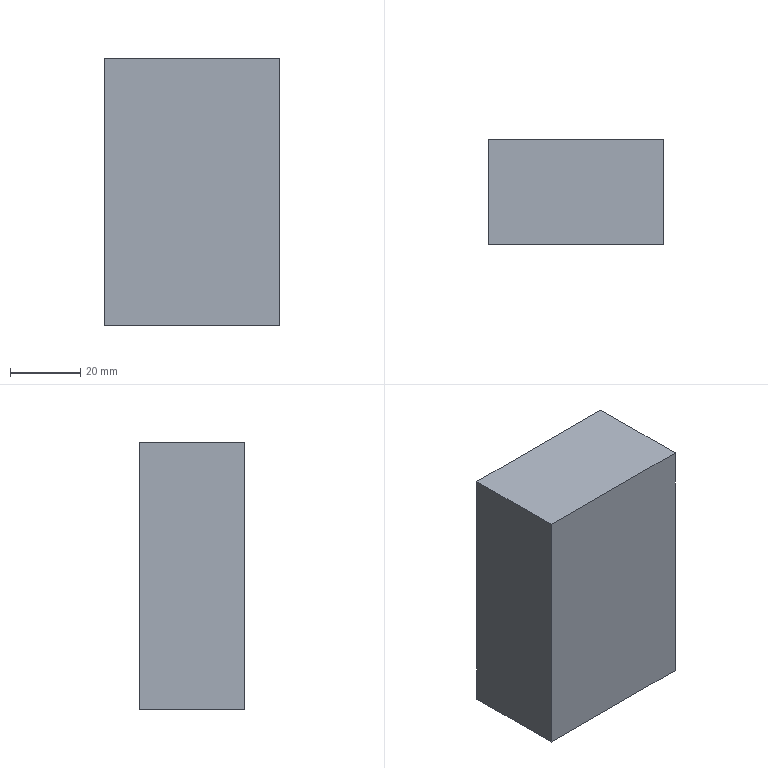Part | SolidWorks | features Extrusion 1 | 1 solid | 6 faces | box 50 x 30 x 76 mm | volume 114000 mm3 | plane 6
STEP:
#1=CARTESIAN_POINT('',(-25.,15.,0.));
#2=VERTEX_POINT('',#1);
#3=CARTESIAN_POINT('',(-25.,-15.,0.));
#4=VERTEX_POINT('',#3);
#5=CARTESIAN_POINT('',(-25.,-15.,0.));
#6=DIRECTION('',(0.,-1.,0.));
#7=VECTOR('',#6,1000.);
#8=LINE('',#5,#7);
#9=EDGE_CURVE('',#2,#4,#8,.T.);
#10=ORIENTED_EDGE('',*,*,#9,.T.);
#11=CARTESIAN_POINT('',(-25.,-15.,76.));
#12=VERTEX_POINT('',#11);
#13=CARTESIAN_POINT('',(-25.,-15.,76.));
#14=DIRECTION('',(0.,0.,-1.));
#15=VECTOR('',#14,1000.);
#16=LINE('',#13,#15);
#17=EDGE_CURVE('',#12,#4,#16,.T.);
#18=ORIENTED_EDGE('',*,*,#17,.F.);
#19=CARTESIAN_POINT('',(-25.,15.,76.));
#20=VERTEX_POINT('',#19);
#21=CARTESIAN_POINT('',(-25.,-15.,76.));
#22=DIRECTION('',(0.,-1.,0.));
#23=VECTOR('',#22,1000.);
#24=LINE('',#21,#23);
#25=EDGE_CURVE('',#20,#12,#24,.T.);
#26=ORIENTED_EDGE('',*,*,#25,.F.);
#27=CARTESIAN_POINT('',(-25.,15.,76.));
#28=DIRECTION('',(0.,0.,-1.));
#29=VECTOR('',#28,1000.);
#30=LINE('',#27,#29);
#31=EDGE_CURVE('',#20,#2,#30,.T.);
#32=ORIENTED_EDGE('',*,*,#31,.T.);
#33=EDGE_LOOP('',(#10,#18,#26,#32));
#34=FACE_OUTER_BOUND('',#33,.T.);
#35=CARTESIAN_POINT('',(-25.,-15.,76.));
#36=DIRECTION('',(1.,0.,0.));
#37=DIRECTION('',(0.,0.,-1.));
#38=AXIS2_PLACEMENT_3D('',#35,#36,#37);
#39=PLANE('',#38);
#40=ADVANCED_FACE('',(#34),#39,.F.);
#41=CARTESIAN_POINT('',(25.,-15.,0.));
#42=VERTEX_POINT('',#41);
#43=CARTESIAN_POINT('',(25.,-15.,0.));
#44=DIRECTION('',(1.,0.,0.));
#45=VECTOR('',#44,1000.);
#46=LINE('',#43,#45);
#47=EDGE_CURVE('',#4,#42,#46,.T.);
#48=ORIENTED_EDGE('',*,*,#47,.T.);
#49=CARTESIAN_POINT('',(25.,-15.,76.));
#50=VERTEX_POINT('',#49);
#51=CARTESIAN_POINT('',(25.,-15.,76.));
#52=DIRECTION('',(0.,0.,-1.));
#53=VECTOR('',#52,1000.);
#54=LINE('',#51,#53);
#55=EDGE_CURVE('',#50,#42,#54,.T.);
#56=ORIENTED_EDGE('',*,*,#55,.F.);
#57=CARTESIAN_POINT('',(25.,-15.,76.));
#58=DIRECTION('',(1.,0.,0.));
#59=VECTOR('',#58,1000.);
#60=LINE('',#57,#59);
#61=EDGE_CURVE('',#12,#50,#60,.T.);
#62=ORIENTED_EDGE('',*,*,#61,.F.);
#63=ORIENTED_EDGE('',*,*,#17,.T.);
#64=EDGE_LOOP('',(#48,#56,#62,#63));
#65=FACE_OUTER_BOUND('',#64,.T.);
#66=CARTESIAN_POINT('',(25.,-15.,76.));
#67=DIRECTION('',(0.,1.,0.));
#68=DIRECTION('',(-1.,0.,0.));
#69=AXIS2_PLACEMENT_3D('',#66,#67,#68);
#70=PLANE('',#69);
#71=ADVANCED_FACE('',(#65),#70,.F.);
#72=CARTESIAN_POINT('',(25.,15.,0.));
#73=VERTEX_POINT('',#72);
#74=CARTESIAN_POINT('',(25.,-15.,0.));
#75=DIRECTION('',(0.,1.,0.));
#76=VECTOR('',#75,1000.);
#77=LINE('',#74,#76);
#78=EDGE_CURVE('',#42,#73,#77,.T.);
#79=ORIENTED_EDGE('',*,*,#78,.T.);
#80=CARTESIAN_POINT('',(25.,15.,76.));
#81=VERTEX_POINT('',#80);
#82=CARTESIAN_POINT('',(25.,15.,76.));
#83=DIRECTION('',(0.,0.,-1.));
#84=VECTOR('',#83,1000.);
#85=LINE('',#82,#84);
#86=EDGE_CURVE('',#81,#73,#85,.T.);
#87=ORIENTED_EDGE('',*,*,#86,.F.);
#88=CARTESIAN_POINT('',(25.,-15.,76.));
#89=DIRECTION('',(0.,1.,0.));
#90=VECTOR('',#89,1000.);
#91=LINE('',#88,#90);
#92=EDGE_CURVE('',#50,#81,#91,.T.);
#93=ORIENTED_EDGE('',*,*,#92,.F.);
#94=ORIENTED_EDGE('',*,*,#55,.T.);
#95=EDGE_LOOP('',(#79,#87,#93,#94));
#96=FACE_OUTER_BOUND('',#95,.T.);
#97=CARTESIAN_POINT('',(25.,-15.,76.));
#98=DIRECTION('',(-1.,0.,0.));
#99=DIRECTION('',(0.,0.,1.));
#100=AXIS2_PLACEMENT_3D('',#97,#98,#99);
#101=PLANE('',#100);
#102=ADVANCED_FACE('',(#96),#101,.F.);
#103=CARTESIAN_POINT('',(25.,15.,0.));
#104=DIRECTION('',(-1.,0.,0.));
#105=VECTOR('',#104,1000.);
#106=LINE('',#103,#105);
#107=EDGE_CURVE('',#73,#2,#106,.T.);
#108=ORIENTED_EDGE('',*,*,#107,.T.);
#109=ORIENTED_EDGE('',*,*,#31,.F.);
#110=CARTESIAN_POINT('',(25.,15.,76.));
#111=DIRECTION('',(-1.,0.,0.));
#112=VECTOR('',#111,1000.);
#113=LINE('',#110,#112);
#114=EDGE_CURVE('',#81,#20,#113,.T.);
#115=ORIENTED_EDGE('',*,*,#114,.F.);
#116=ORIENTED_EDGE('',*,*,#86,.T.);
#117=EDGE_LOOP('',(#108,#109,#115,#116));
#118=FACE_OUTER_BOUND('',#117,.T.);
#119=CARTESIAN_POINT('',(25.,15.,76.));
#120=DIRECTION('',(0.,-1.,0.));
#121=DIRECTION('',(1.,0.,0.));
#122=AXIS2_PLACEMENT_3D('',#119,#120,#121);
#123=PLANE('',#122);
#124=ADVANCED_FACE('',(#118),#123,.F.);
#125=ORIENTED_EDGE('',*,*,#25,.T.);
#126=ORIENTED_EDGE('',*,*,#61,.T.);
#127=ORIENTED_EDGE('',*,*,#92,.T.);
#128=ORIENTED_EDGE('',*,*,#114,.T.);
#129=EDGE_LOOP('',(#125,#126,#127,#128));
#130=FACE_OUTER_BOUND('',#129,.T.);
#131=CARTESIAN_POINT('',(0.,0.,76.));
#132=DIRECTION('',(0.,0.,1.));
#133=DIRECTION('',(1.,0.,0.));
#134=AXIS2_PLACEMENT_3D('',#131,#132,#133);
#135=PLANE('',#134);
#136=ADVANCED_FACE('',(#130),#135,.T.);
#137=ORIENTED_EDGE('',*,*,#9,.F.);
#138=ORIENTED_EDGE('',*,*,#107,.F.);
#139=ORIENTED_EDGE('',*,*,#78,.F.);
#140=ORIENTED_EDGE('',*,*,#47,.F.);
#141=EDGE_LOOP('',(#137,#138,#139,#140));
#142=FACE_OUTER_BOUND('',#141,.T.);
#143=CARTESIAN_POINT('',(0.,0.,0.));
#144=DIRECTION('',(0.,0.,1.));
#145=DIRECTION('',(1.,0.,0.));
#146=AXIS2_PLACEMENT_3D('',#143,#144,#145);
#147=PLANE('',#146);
#148=ADVANCED_FACE('',(#142),#147,.F.);
#149=CLOSED_SHELL('',(#40,#71,#102,#124,#136,#148));
#150=MANIFOLD_SOLID_BREP('',#149);
#151=CARTESIAN_POINT('',(0.,0.,0.));
#152=DIRECTION('',(0.,0.,1.));
#153=DIRECTION('',(1.,0.,0.));
#154=AXIS2_PLACEMENT_3D('',#151,#152,#153);
#155=(LENGTH_UNIT()NAMED_UNIT(*)SI_UNIT(.MILLI.,.METRE.));
#156=UNCERTAINTY_MEASURE_WITH_UNIT(LENGTH_MEASURE(0.00001),#155,'','');
#157=(NAMED_UNIT(*)PLANE_ANGLE_UNIT()SI_UNIT($,.RADIAN.));
#158=(NAMED_UNIT(*)SI_UNIT($,.STERADIAN.)SOLID_ANGLE_UNIT());
#159=(GEOMETRIC_REPRESENTATION_CONTEXT(3)GLOBAL_UNCERTAINTY_ASSIGNED_CONTEXT((#156))GLOBAL_UNIT_ASSIGNED_CONTEXT((#155,#157,#158))REPRESENTATION_CONTEXT('',''));
#160=ADVANCED_BREP_SHAPE_REPRESENTATION('',(#150,#154),#159);